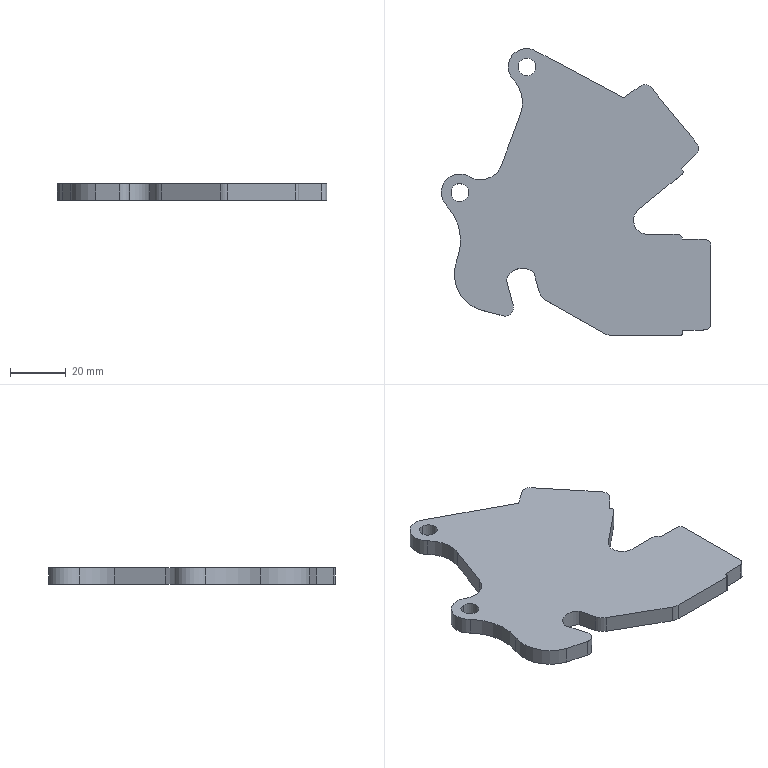Part | STEP file | PRT0001_68_2 | 1 solid | 42 faces | box 96.462 x 102.711 x 6 mm | volume 37428 mm3 | cylinder 22 | plane 20 | commonest cylinder face diameters 6.324 x4 4 x3 6 x3 10 x3 2 x2 12 x1